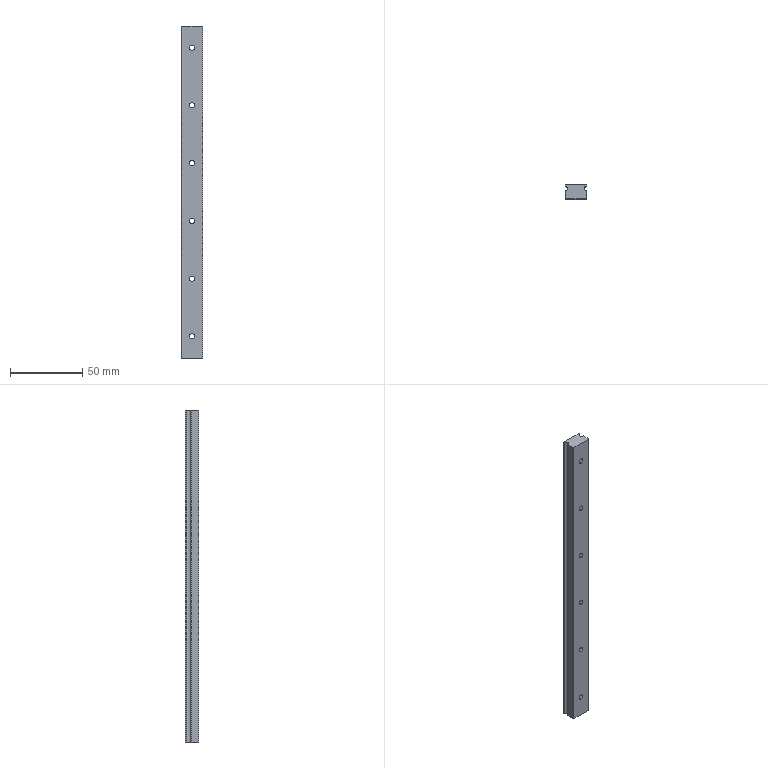Part | STEP file | 1SE2BZ16-230 | 1 solid | 43 faces | box 15 x 9.5 x 230 mm | volume 29723 mm3 | cylinder 27 | plane 16 | commonest cylinder face diameters 3.5 x12 6 x12 3.28 x3